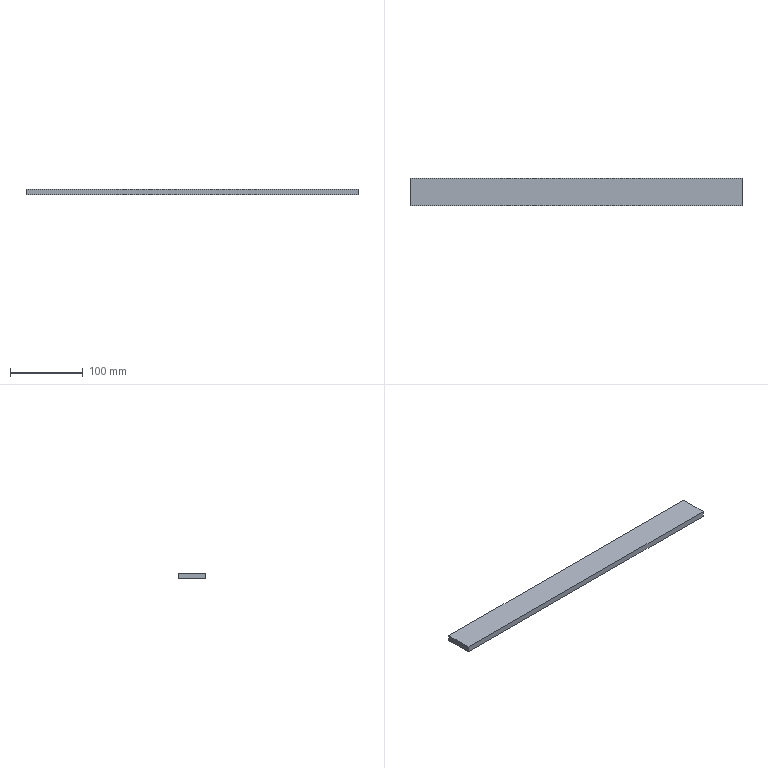Part | STEP file | 124_id1014_x_t | 1 solid | 6 faces | box 455.2 x 38 x 8 mm | volume 138381 mm3 | plane 6
STEP:
#1=CARTESIAN_POINT('',(0.,0.,0.));
#2=DIRECTION('',(0.,0.,1.));
#3=DIRECTION('',(1.,0.,0.));
#4=AXIS2_PLACEMENT_3D('',#1,#2,#3);
#5=CARTESIAN_POINT('',(-250.6,671.25,110.));
#6=VERTEX_POINT('',#5);
#7=CARTESIAN_POINT('',(-705.8,671.25,110.));
#8=VERTEX_POINT('',#7);
#9=CARTESIAN_POINT('',(-478.2,671.25,110.));
#10=DIRECTION('',(-1.,0.,0.));
#11=VECTOR('',#10,1.);
#12=LINE('',#9,#11);
#13=CARTESIAN_POINT('',(-478.2,690.25,110.));
#14=DIRECTION('',(0.,0.,1.));
#15=DIRECTION('',(1.,0.,0.));
#16=AXIS2_PLACEMENT_3D('',#13,#14,#15);
#17=PLANE('',#16);
#18=CARTESIAN_POINT('',(0.,-19.));
#19=DIRECTION('',(-1.,0.));
#20=VECTOR('',#19,1.);
#21=LINE('',#18,#20);
#22=(GEOMETRIC_REPRESENTATION_CONTEXT(2)PARAMETRIC_REPRESENTATION_CONTEXT()REPRESENTATION_CONTEXT('',''));
#23=DEFINITIONAL_REPRESENTATION('',(#21),#22);
#24=PCURVE('',#17,#23);
#25=CARTESIAN_POINT('',(-478.2,671.25,102.));
#26=DIRECTION('',(0.,-1.,0.));
#27=DIRECTION('',(0.,0.,-1.));
#28=AXIS2_PLACEMENT_3D('',#25,#26,#27);
#29=PLANE('',#28);
#30=CARTESIAN_POINT('',(-8.,0.));
#31=DIRECTION('',(0.,-1.));
#32=VECTOR('',#31,1.);
#33=LINE('',#30,#32);
#34=(GEOMETRIC_REPRESENTATION_CONTEXT(2)PARAMETRIC_REPRESENTATION_CONTEXT()REPRESENTATION_CONTEXT('',''));
#35=DEFINITIONAL_REPRESENTATION('',(#33),#34);
#36=PCURVE('',#29,#35);
#37=SURFACE_CURVE('',#12,(#24,#36),.PCURVE_S1.);
#38=EDGE_CURVE('',#6,#8,#37,.T.);
#39=ORIENTED_EDGE('',*,*,#38,.F.);
#40=CARTESIAN_POINT('',(-250.6,709.25,110.));
#41=VERTEX_POINT('',#40);
#42=CARTESIAN_POINT('',(-250.6,690.25,110.));
#43=DIRECTION('',(0.,-1.,0.));
#44=VECTOR('',#43,1.);
#45=LINE('',#42,#44);
#46=CARTESIAN_POINT('',(227.6,0.));
#47=DIRECTION('',(0.,-1.));
#48=VECTOR('',#47,1.);
#49=LINE('',#46,#48);
#50=(GEOMETRIC_REPRESENTATION_CONTEXT(2)PARAMETRIC_REPRESENTATION_CONTEXT()REPRESENTATION_CONTEXT('',''));
#51=DEFINITIONAL_REPRESENTATION('',(#49),#50);
#52=PCURVE('',#17,#51);
#53=CARTESIAN_POINT('',(-250.6,690.25,102.));
#54=DIRECTION('',(1.,0.,0.));
#55=DIRECTION('',(0.,0.,-1.));
#56=AXIS2_PLACEMENT_3D('',#53,#54,#55);
#57=PLANE('',#56);
#58=CARTESIAN_POINT('',(-8.,0.));
#59=DIRECTION('',(0.,-1.));
#60=VECTOR('',#59,1.);
#61=LINE('',#58,#60);
#62=(GEOMETRIC_REPRESENTATION_CONTEXT(2)PARAMETRIC_REPRESENTATION_CONTEXT()REPRESENTATION_CONTEXT('',''));
#63=DEFINITIONAL_REPRESENTATION('',(#61),#62);
#64=PCURVE('',#57,#63);
#65=SURFACE_CURVE('',#45,(#52,#64),.PCURVE_S1.);
#66=EDGE_CURVE('',#41,#6,#65,.T.);
#67=ORIENTED_EDGE('',*,*,#66,.F.);
#68=CARTESIAN_POINT('',(-705.8,709.25,110.));
#69=VERTEX_POINT('',#68);
#70=CARTESIAN_POINT('',(-478.2,709.25,110.));
#71=DIRECTION('',(1.,0.,0.));
#72=VECTOR('',#71,1.);
#73=LINE('',#70,#72);
#74=CARTESIAN_POINT('',(0.,19.));
#75=DIRECTION('',(1.,0.));
#76=VECTOR('',#75,1.);
#77=LINE('',#74,#76);
#78=(GEOMETRIC_REPRESENTATION_CONTEXT(2)PARAMETRIC_REPRESENTATION_CONTEXT()REPRESENTATION_CONTEXT('',''));
#79=DEFINITIONAL_REPRESENTATION('',(#77),#78);
#80=PCURVE('',#17,#79);
#81=CARTESIAN_POINT('',(-478.2,709.25,102.));
#82=DIRECTION('',(0.,1.,0.));
#83=DIRECTION('',(0.,0.,1.));
#84=AXIS2_PLACEMENT_3D('',#81,#82,#83);
#85=PLANE('',#84);
#86=CARTESIAN_POINT('',(8.,0.));
#87=DIRECTION('',(0.,1.));
#88=VECTOR('',#87,1.);
#89=LINE('',#86,#88);
#90=(GEOMETRIC_REPRESENTATION_CONTEXT(2)PARAMETRIC_REPRESENTATION_CONTEXT()REPRESENTATION_CONTEXT('',''));
#91=DEFINITIONAL_REPRESENTATION('',(#89),#90);
#92=PCURVE('',#85,#91);
#93=SURFACE_CURVE('',#73,(#80,#92),.PCURVE_S1.);
#94=EDGE_CURVE('',#69,#41,#93,.T.);
#95=ORIENTED_EDGE('',*,*,#94,.F.);
#96=CARTESIAN_POINT('',(-705.8,690.25,110.));
#97=DIRECTION('',(0.,1.,0.));
#98=VECTOR('',#97,1.);
#99=LINE('',#96,#98);
#100=CARTESIAN_POINT('',(-227.6,0.));
#101=DIRECTION('',(0.,1.));
#102=VECTOR('',#101,1.);
#103=LINE('',#100,#102);
#104=(GEOMETRIC_REPRESENTATION_CONTEXT(2)PARAMETRIC_REPRESENTATION_CONTEXT()REPRESENTATION_CONTEXT('',''));
#105=DEFINITIONAL_REPRESENTATION('',(#103),#104);
#106=PCURVE('',#17,#105);
#107=CARTESIAN_POINT('',(-705.8,690.25,102.));
#108=DIRECTION('',(-1.,0.,0.));
#109=DIRECTION('',(0.,0.,1.));
#110=AXIS2_PLACEMENT_3D('',#107,#108,#109);
#111=PLANE('',#110);
#112=CARTESIAN_POINT('',(8.,0.));
#113=DIRECTION('',(0.,1.));
#114=VECTOR('',#113,1.);
#115=LINE('',#112,#114);
#116=(GEOMETRIC_REPRESENTATION_CONTEXT(2)PARAMETRIC_REPRESENTATION_CONTEXT()REPRESENTATION_CONTEXT('',''));
#117=DEFINITIONAL_REPRESENTATION('',(#115),#116);
#118=PCURVE('',#111,#117);
#119=SURFACE_CURVE('',#99,(#106,#118),.PCURVE_S1.);
#120=EDGE_CURVE('',#8,#69,#119,.T.);
#121=ORIENTED_EDGE('',*,*,#120,.F.);
#122=EDGE_LOOP('',(#39,#67,#95,#121));
#123=FACE_BOUND('',#122,.T.);
#124=ADVANCED_FACE('',(#123),#17,.T.);
#125=CARTESIAN_POINT('',(-250.6,671.25,102.));
#126=VERTEX_POINT('',#125);
#127=CARTESIAN_POINT('',(-250.6,671.25,102.));
#128=DIRECTION('',(0.,0.,1.));
#129=VECTOR('',#128,1.);
#130=LINE('',#127,#129);
#131=CARTESIAN_POINT('',(0.,227.6));
#132=DIRECTION('',(-1.,0.));
#133=VECTOR('',#132,1.);
#134=LINE('',#131,#133);
#135=(GEOMETRIC_REPRESENTATION_CONTEXT(2)PARAMETRIC_REPRESENTATION_CONTEXT()REPRESENTATION_CONTEXT('',''));
#136=DEFINITIONAL_REPRESENTATION('',(#134),#135);
#137=PCURVE('',#29,#136);
#138=CARTESIAN_POINT('',(0.,-19.));
#139=DIRECTION('',(-1.,0.));
#140=VECTOR('',#139,1.);
#141=LINE('',#138,#140);
#142=(GEOMETRIC_REPRESENTATION_CONTEXT(2)PARAMETRIC_REPRESENTATION_CONTEXT()REPRESENTATION_CONTEXT('',''));
#143=DEFINITIONAL_REPRESENTATION('',(#141),#142);
#144=PCURVE('',#57,#143);
#145=SURFACE_CURVE('',#130,(#137,#144),.PCURVE_S1.);
#146=EDGE_CURVE('',#126,#6,#145,.T.);
#147=ORIENTED_EDGE('',*,*,#146,.T.);
#148=ORIENTED_EDGE('',*,*,#38,.T.);
#149=CARTESIAN_POINT('',(-705.8,671.25,102.));
#150=VERTEX_POINT('',#149);
#151=CARTESIAN_POINT('',(-705.8,671.25,102.));
#152=DIRECTION('',(0.,0.,1.));
#153=VECTOR('',#152,1.);
#154=LINE('',#151,#153);
#155=CARTESIAN_POINT('',(0.,-227.6));
#156=DIRECTION('',(-1.,0.));
#157=VECTOR('',#156,1.);
#158=LINE('',#155,#157);
#159=(GEOMETRIC_REPRESENTATION_CONTEXT(2)PARAMETRIC_REPRESENTATION_CONTEXT()REPRESENTATION_CONTEXT('',''));
#160=DEFINITIONAL_REPRESENTATION('',(#158),#159);
#161=PCURVE('',#29,#160);
#162=CARTESIAN_POINT('',(0.,-19.));
#163=DIRECTION('',(1.,0.));
#164=VECTOR('',#163,1.);
#165=LINE('',#162,#164);
#166=(GEOMETRIC_REPRESENTATION_CONTEXT(2)PARAMETRIC_REPRESENTATION_CONTEXT()REPRESENTATION_CONTEXT('',''));
#167=DEFINITIONAL_REPRESENTATION('',(#165),#166);
#168=PCURVE('',#111,#167);
#169=SURFACE_CURVE('',#154,(#161,#168),.PCURVE_S1.);
#170=EDGE_CURVE('',#150,#8,#169,.T.);
#171=ORIENTED_EDGE('',*,*,#170,.F.);
#172=CARTESIAN_POINT('',(-478.2,671.25,102.));
#173=DIRECTION('',(1.,0.,0.));
#174=VECTOR('',#173,1.);
#175=LINE('',#172,#174);
#176=CARTESIAN_POINT('',(0.,0.));
#177=DIRECTION('',(0.,1.));
#178=VECTOR('',#177,1.);
#179=LINE('',#176,#178);
#180=(GEOMETRIC_REPRESENTATION_CONTEXT(2)PARAMETRIC_REPRESENTATION_CONTEXT()REPRESENTATION_CONTEXT('',''));
#181=DEFINITIONAL_REPRESENTATION('',(#179),#180);
#182=PCURVE('',#29,#181);
#183=CARTESIAN_POINT('',(-478.2,690.25,102.));
#184=DIRECTION('',(0.,0.,-1.));
#185=DIRECTION('',(-1.,0.,0.));
#186=AXIS2_PLACEMENT_3D('',#183,#184,#185);
#187=PLANE('',#186);
#188=CARTESIAN_POINT('',(0.,-19.));
#189=DIRECTION('',(-1.,0.));
#190=VECTOR('',#189,1.);
#191=LINE('',#188,#190);
#192=(GEOMETRIC_REPRESENTATION_CONTEXT(2)PARAMETRIC_REPRESENTATION_CONTEXT()REPRESENTATION_CONTEXT('',''));
#193=DEFINITIONAL_REPRESENTATION('',(#191),#192);
#194=PCURVE('',#187,#193);
#195=SURFACE_CURVE('',#175,(#182,#194),.PCURVE_S1.);
#196=EDGE_CURVE('',#150,#126,#195,.T.);
#197=ORIENTED_EDGE('',*,*,#196,.T.);
#198=EDGE_LOOP('',(#147,#148,#171,#197));
#199=FACE_BOUND('',#198,.T.);
#200=ADVANCED_FACE('',(#199),#29,.T.);
#201=ORIENTED_EDGE('',*,*,#170,.T.);
#202=ORIENTED_EDGE('',*,*,#120,.T.);
#203=CARTESIAN_POINT('',(-705.8,709.25,102.));
#204=VERTEX_POINT('',#203);
#205=CARTESIAN_POINT('',(-705.8,709.25,102.));
#206=DIRECTION('',(0.,0.,1.));
#207=VECTOR('',#206,1.);
#208=LINE('',#205,#207);
#209=CARTESIAN_POINT('',(0.,19.));
#210=DIRECTION('',(1.,0.));
#211=VECTOR('',#210,1.);
#212=LINE('',#209,#211);
#213=(GEOMETRIC_REPRESENTATION_CONTEXT(2)PARAMETRIC_REPRESENTATION_CONTEXT()REPRESENTATION_CONTEXT('',''));
#214=DEFINITIONAL_REPRESENTATION('',(#212),#213);
#215=PCURVE('',#111,#214);
#216=CARTESIAN_POINT('',(0.,-227.6));
#217=DIRECTION('',(1.,0.));
#218=VECTOR('',#217,1.);
#219=LINE('',#216,#218);
#220=(GEOMETRIC_REPRESENTATION_CONTEXT(2)PARAMETRIC_REPRESENTATION_CONTEXT()REPRESENTATION_CONTEXT('',''));
#221=DEFINITIONAL_REPRESENTATION('',(#219),#220);
#222=PCURVE('',#85,#221);
#223=SURFACE_CURVE('',#208,(#215,#222),.PCURVE_S1.);
#224=EDGE_CURVE('',#204,#69,#223,.T.);
#225=ORIENTED_EDGE('',*,*,#224,.F.);
#226=CARTESIAN_POINT('',(-705.8,690.25,102.));
#227=DIRECTION('',(0.,-1.,0.));
#228=VECTOR('',#227,1.);
#229=LINE('',#226,#228);
#230=CARTESIAN_POINT('',(0.,0.));
#231=DIRECTION('',(0.,-1.));
#232=VECTOR('',#231,1.);
#233=LINE('',#230,#232);
#234=(GEOMETRIC_REPRESENTATION_CONTEXT(2)PARAMETRIC_REPRESENTATION_CONTEXT()REPRESENTATION_CONTEXT('',''));
#235=DEFINITIONAL_REPRESENTATION('',(#233),#234);
#236=PCURVE('',#111,#235);
#237=CARTESIAN_POINT('',(227.6,0.));
#238=DIRECTION('',(0.,-1.));
#239=VECTOR('',#238,1.);
#240=LINE('',#237,#239);
#241=(GEOMETRIC_REPRESENTATION_CONTEXT(2)PARAMETRIC_REPRESENTATION_CONTEXT()REPRESENTATION_CONTEXT('',''));
#242=DEFINITIONAL_REPRESENTATION('',(#240),#241);
#243=PCURVE('',#187,#242);
#244=SURFACE_CURVE('',#229,(#236,#243),.PCURVE_S1.);
#245=EDGE_CURVE('',#204,#150,#244,.T.);
#246=ORIENTED_EDGE('',*,*,#245,.T.);
#247=EDGE_LOOP('',(#201,#202,#225,#246));
#248=FACE_BOUND('',#247,.T.);
#249=ADVANCED_FACE('',(#248),#111,.T.);
#250=ORIENTED_EDGE('',*,*,#224,.T.);
#251=ORIENTED_EDGE('',*,*,#94,.T.);
#252=CARTESIAN_POINT('',(-250.6,709.25,102.));
#253=VERTEX_POINT('',#252);
#254=CARTESIAN_POINT('',(-250.6,709.25,102.));
#255=DIRECTION('',(0.,0.,1.));
#256=VECTOR('',#255,1.);
#257=LINE('',#254,#256);
#258=CARTESIAN_POINT('',(0.,227.6));
#259=DIRECTION('',(1.,0.));
#260=VECTOR('',#259,1.);
#261=LINE('',#258,#260);
#262=(GEOMETRIC_REPRESENTATION_CONTEXT(2)PARAMETRIC_REPRESENTATION_CONTEXT()REPRESENTATION_CONTEXT('',''));
#263=DEFINITIONAL_REPRESENTATION('',(#261),#262);
#264=PCURVE('',#85,#263);
#265=CARTESIAN_POINT('',(0.,19.));
#266=DIRECTION('',(-1.,0.));
#267=VECTOR('',#266,1.);
#268=LINE('',#265,#267);
#269=(GEOMETRIC_REPRESENTATION_CONTEXT(2)PARAMETRIC_REPRESENTATION_CONTEXT()REPRESENTATION_CONTEXT('',''));
#270=DEFINITIONAL_REPRESENTATION('',(#268),#269);
#271=PCURVE('',#57,#270);
#272=SURFACE_CURVE('',#257,(#264,#271),.PCURVE_S1.);
#273=EDGE_CURVE('',#253,#41,#272,.T.);
#274=ORIENTED_EDGE('',*,*,#273,.F.);
#275=CARTESIAN_POINT('',(-478.2,709.25,102.));
#276=DIRECTION('',(-1.,0.,0.));
#277=VECTOR('',#276,1.);
#278=LINE('',#275,#277);
#279=CARTESIAN_POINT('',(0.,0.));
#280=DIRECTION('',(0.,-1.));
#281=VECTOR('',#280,1.);
#282=LINE('',#279,#281);
#283=(GEOMETRIC_REPRESENTATION_CONTEXT(2)PARAMETRIC_REPRESENTATION_CONTEXT()REPRESENTATION_CONTEXT('',''));
#284=DEFINITIONAL_REPRESENTATION('',(#282),#283);
#285=PCURVE('',#85,#284);
#286=CARTESIAN_POINT('',(0.,19.));
#287=DIRECTION('',(1.,0.));
#288=VECTOR('',#287,1.);
#289=LINE('',#286,#288);
#290=(GEOMETRIC_REPRESENTATION_CONTEXT(2)PARAMETRIC_REPRESENTATION_CONTEXT()REPRESENTATION_CONTEXT('',''));
#291=DEFINITIONAL_REPRESENTATION('',(#289),#290);
#292=PCURVE('',#187,#291);
#293=SURFACE_CURVE('',#278,(#285,#292),.PCURVE_S1.);
#294=EDGE_CURVE('',#253,#204,#293,.T.);
#295=ORIENTED_EDGE('',*,*,#294,.T.);
#296=EDGE_LOOP('',(#250,#251,#274,#295));
#297=FACE_BOUND('',#296,.T.);
#298=ADVANCED_FACE('',(#297),#85,.T.);
#299=CARTESIAN_POINT('',(-250.6,690.25,102.));
#300=DIRECTION('',(0.,1.,0.));
#301=VECTOR('',#300,1.);
#302=LINE('',#299,#301);
#303=CARTESIAN_POINT('',(-227.6,0.));
#304=DIRECTION('',(0.,1.));
#305=VECTOR('',#304,1.);
#306=LINE('',#303,#305);
#307=(GEOMETRIC_REPRESENTATION_CONTEXT(2)PARAMETRIC_REPRESENTATION_CONTEXT()REPRESENTATION_CONTEXT('',''));
#308=DEFINITIONAL_REPRESENTATION('',(#306),#307);
#309=PCURVE('',#187,#308);
#310=CARTESIAN_POINT('',(0.,0.));
#311=DIRECTION('',(0.,1.));
#312=VECTOR('',#311,1.);
#313=LINE('',#310,#312);
#314=(GEOMETRIC_REPRESENTATION_CONTEXT(2)PARAMETRIC_REPRESENTATION_CONTEXT()REPRESENTATION_CONTEXT('',''));
#315=DEFINITIONAL_REPRESENTATION('',(#313),#314);
#316=PCURVE('',#57,#315);
#317=SURFACE_CURVE('',#302,(#309,#316),.PCURVE_S1.);
#318=EDGE_CURVE('',#126,#253,#317,.T.);
#319=ORIENTED_EDGE('',*,*,#318,.F.);
#320=ORIENTED_EDGE('',*,*,#196,.F.);
#321=ORIENTED_EDGE('',*,*,#245,.F.);
#322=ORIENTED_EDGE('',*,*,#294,.F.);
#323=EDGE_LOOP('',(#319,#320,#321,#322));
#324=FACE_BOUND('',#323,.T.);
#325=ADVANCED_FACE('',(#324),#187,.T.);
#326=ORIENTED_EDGE('',*,*,#318,.T.);
#327=ORIENTED_EDGE('',*,*,#273,.T.);
#328=ORIENTED_EDGE('',*,*,#66,.T.);
#329=ORIENTED_EDGE('',*,*,#146,.F.);
#330=EDGE_LOOP('',(#326,#327,#328,#329));
#331=FACE_BOUND('',#330,.T.);
#332=ADVANCED_FACE('',(#331),#57,.T.);
#333=CLOSED_SHELL('',(#124,#200,#249,#298,#325,#332));
#334=MANIFOLD_SOLID_BREP('',#333);
#335=(LENGTH_UNIT()NAMED_UNIT(*)SI_UNIT(.MILLI.,.METRE.));
#336=UNCERTAINTY_MEASURE_WITH_UNIT(LENGTH_MEASURE(0.0000001),#335,'','');
#337=(NAMED_UNIT(*)PLANE_ANGLE_UNIT()SI_UNIT($,.RADIAN.));
#338=(NAMED_UNIT(*)SI_UNIT($,.STERADIAN.)SOLID_ANGLE_UNIT());
#339=(GEOMETRIC_REPRESENTATION_CONTEXT(3)GLOBAL_UNCERTAINTY_ASSIGNED_CONTEXT((#336))GLOBAL_UNIT_ASSIGNED_CONTEXT((#335,#337,#338))REPRESENTATION_CONTEXT('',''));
#340=ADVANCED_BREP_SHAPE_REPRESENTATION('',(#4,#334),#339);